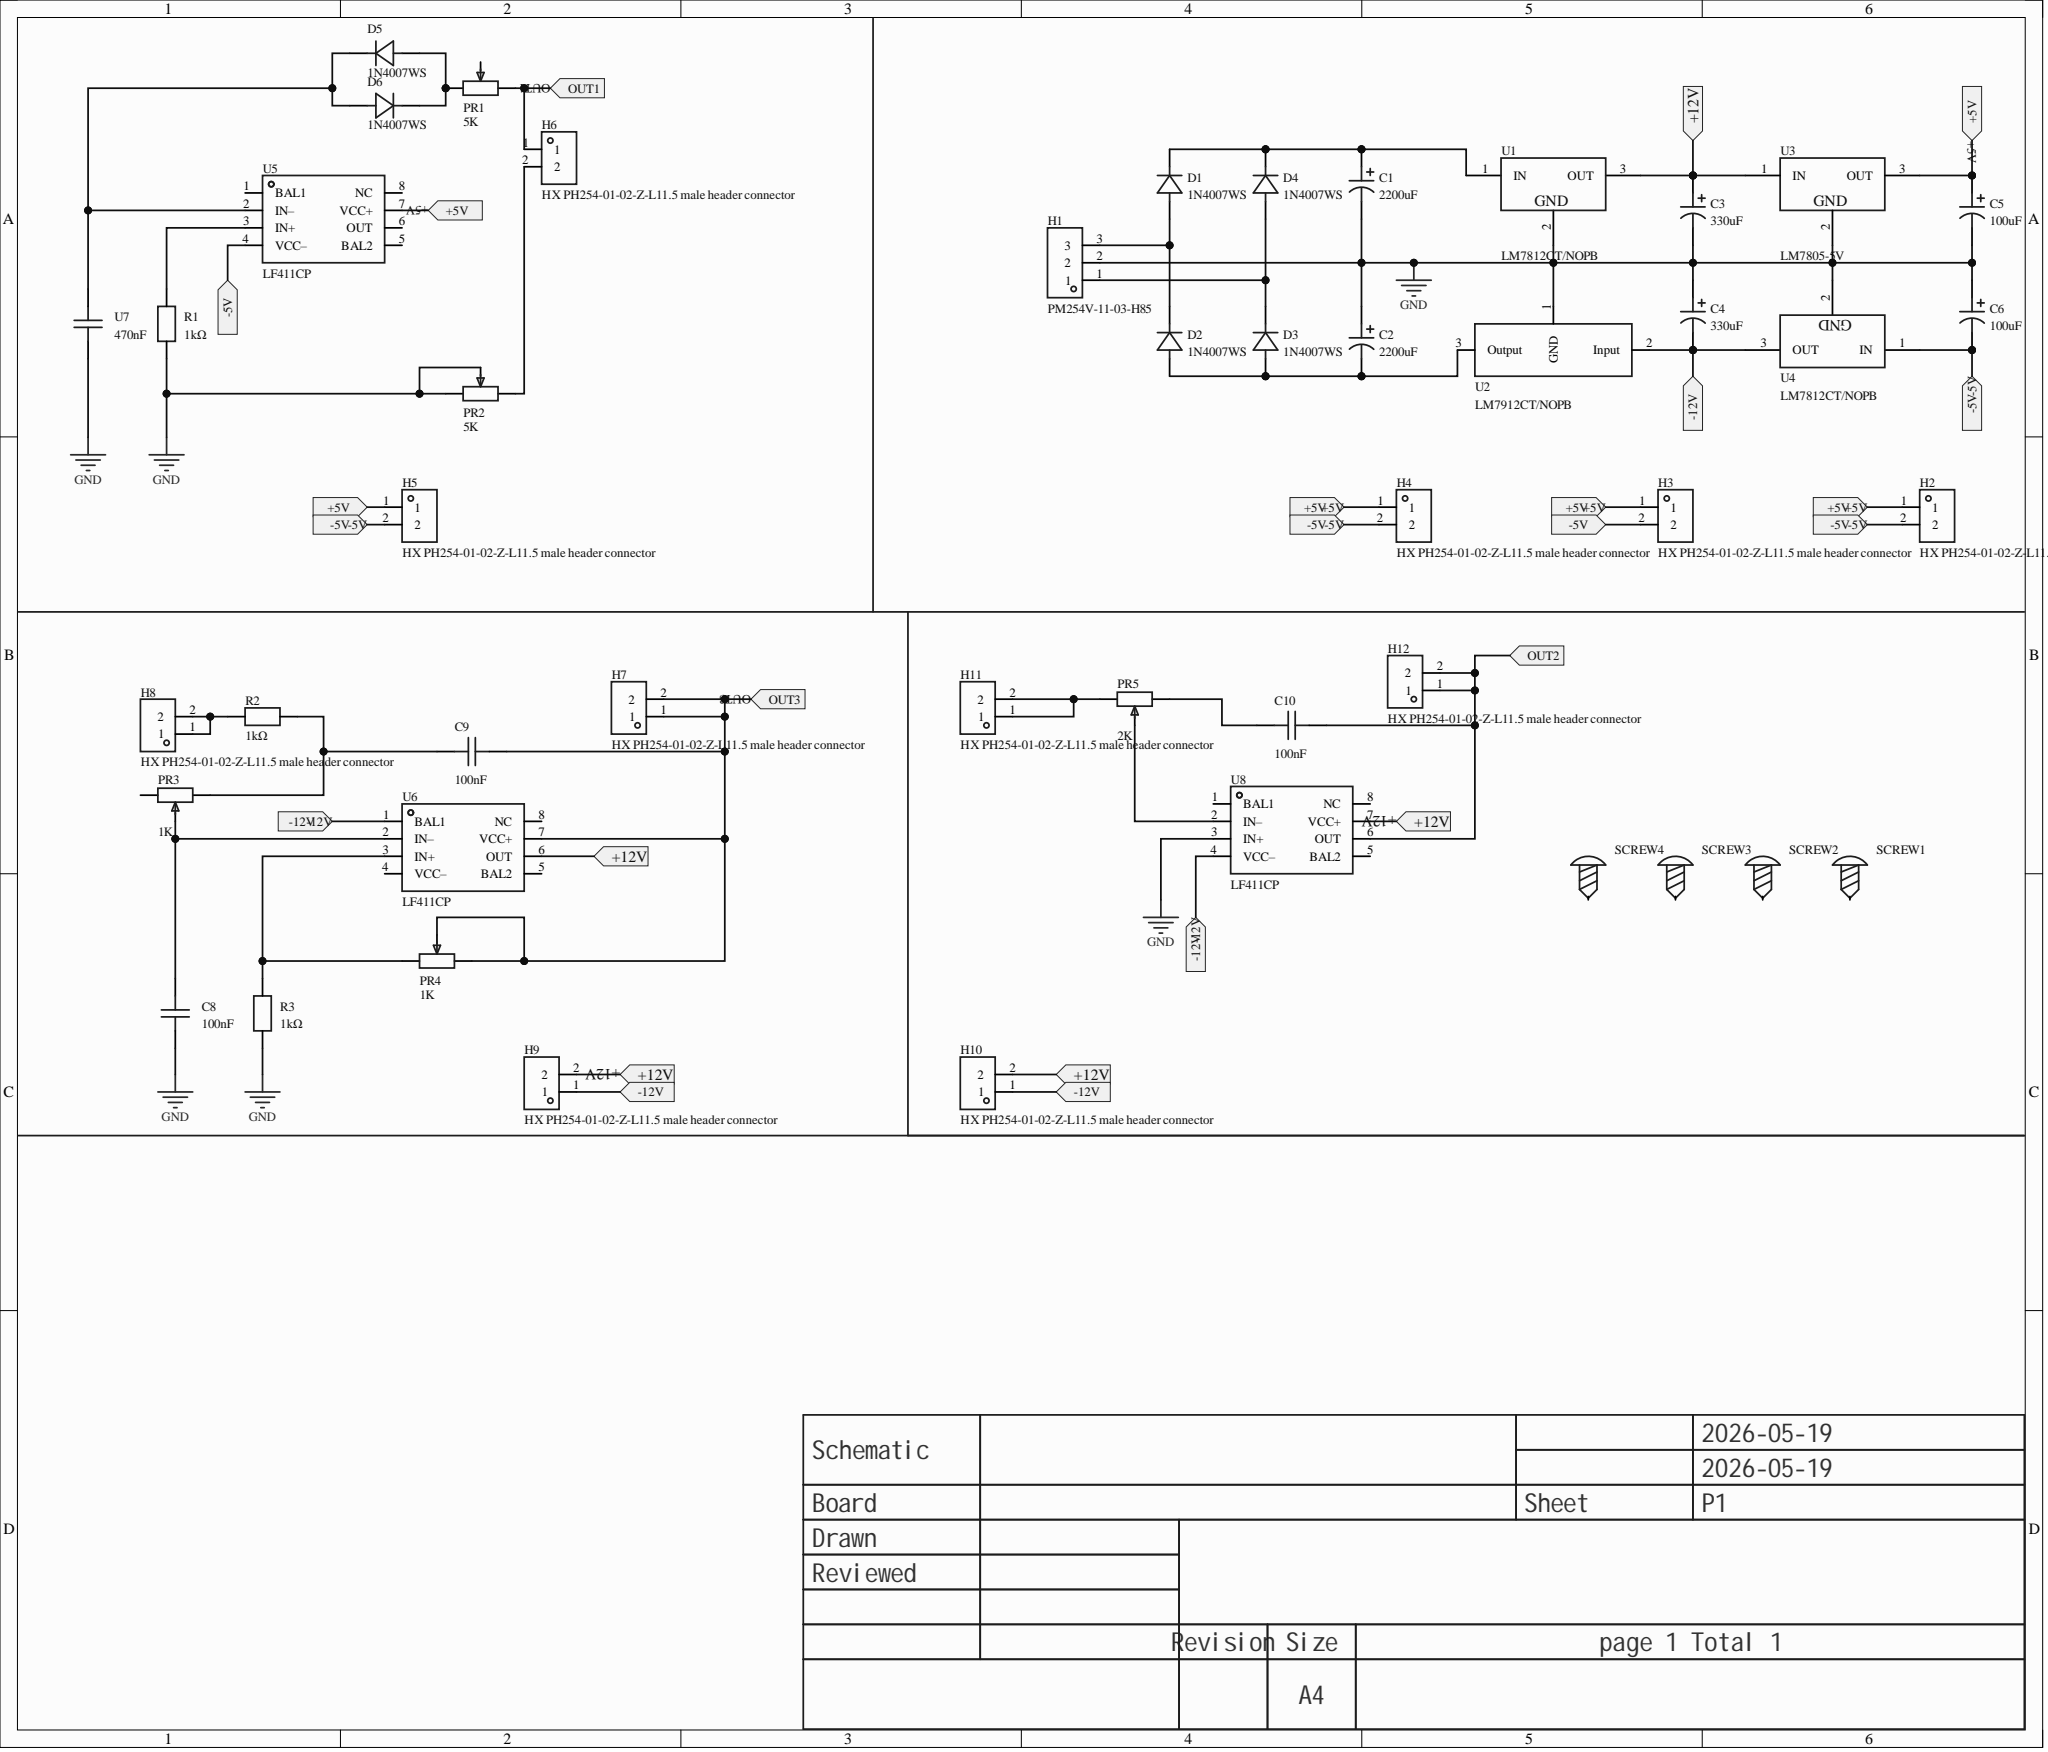Circuit board | Altium Designer | 47 parts | 23 nets
Bill of materials:
Comment,Description,Designator,Footprint,LibRef,Quantity
"2200uF","Capacitance:2200uF;Tolerance:±20%;Rated voltage:35V;","C1, C2","CAP-TH_BD16.0-P7.50-D0.8-FD","ERA35V2200M16X26","2"
"330uF","Capacitance:330uF;Tolerance:±20%;Rated voltage:16V;Ripple current:105mA@120Hz;Equivalent series resistance (ESR):-;","C3, C4","CAP-SMD_BD6.3-L6.6-W6.6-LS7.2-FD_3","RVT16V330M6X8","2"
"100uF","Capacitance:100uF;Tolerance:±20%;Rated voltage:50V;Ripple current:140mA@120Hz;","C5, C6","CAP-SMD_BD6.3-L6.6-W6.6-LS7.3-FD-H7.7","JVJ50V100M6x8","2"
"100nF","Capacitance:100nF;Tolerance:-20%~+80%;Rated voltage:50V;Temperature coefficient:Y5V;","C8, C9, C10","CAP-TH_L5.0-W2.5-P2.54-D0.7","CC1H104ZA1PD3F5P3003","3"
"1N4007WS","Diode configuration:1 single unit;Forward voltage (Vf):1.1V@1A;DC reverse voltage (Vr):1kV;Rectified current:1A;","D1, D2, D3, D4, D5, D6","SOD-323_L1.7-W1.3-LS2.5-RD","1N4007WS_C53055759","6"
"PM254V-11-03-H85","Socket structure:1x3P;Pitch:2.54mm;Row spacing:-;Round/square hole:Square hole;Mounting:Through-hole;Rows:Single row;Total holes:3P;Rated current:3A;Socket direction:Top;Plastic height:8.5mm;Contact material:Brass;Contact plating:-;Operating temperature:-40℃~+105℃;","H1","HDR-TH_3P-P2.54-V-F","PM254V-11-03-H85","1"
"HX PH254-01-02-Z-L11.5 male header connector","Pin structure:1x2P;Pitch:2.54mm;Round/square pin:Square pin;Mounting:Through-hole;Rows:Single row;Total pins:2P;Rated current:3A;Rated voltage:1kV;Mating pin length:6mm;Plastic height:2.5mm;Termination pin length:3mm;Contact material:Brass;Contact plating:Gold;Operating temperature:-40℃~+105℃;","H2, H3, H4, H5, H6, H7, H8, H9, H10, H11, H12","HDR-TH_2P-P2.54-V-M","HX PH254-01-02-Z-L11.5 male header connector","11"
"5K","","PR1, PR2","R_3386P","R_3386P","2"
"1K","","PR3, PR4","R_3386P","R_3386P","2"
"2K","","PR5","R_3386P","R_3386P","1"
"1kΩ","Resistor type:Thick film resistor;Resistance:1kΩ;Tolerance:±0.1%;Power:100mW;Working voltage:75V;Temperature coefficient:±100ppm/?;","R1, R2, R3","R0603","FRH0603B1001TS","3"
"","","SCREW1, SCREW2, SCREW3, SCREW4","M2螺丝","M2螺丝","4"
"LM7812CT/NOPB","Output type:Fixed;Max input voltage:-;Output voltage:12V;Output current:1.5A;Power supply rejection ratio (PSRR):72dB@(120Hz);Output polarity:Positive;","U1, U4","TO-220-3_L10.2-W4.6-P2.54-L","LM7812CT/NOPB","2"
"LM7912CT/NOPB","Output type:Fixed;Max input voltage:35V;Output voltage:12V;Output current:1.5A;Power supply rejection ratio (PSRR):70dB@(120Hz);Output polarity:Negative;","U2","TO-220-3_L10.2-W4.6-P2.54-L","LM7912CT/NOPB","1"
"LM7805-5V","","U3","TO-252-2_L6.6-W6.1-P4.58-LS9.9-TL","LM7805-5V_C9900008050","1"
"LF411CP","Gain-bandwidth product (GBP):3MHz;Input bias current (Ib):50pA;Input offset voltage (Vos):800uV;Slew rate (SR):13V/us;","U5, U6, U8","PDIP-8_L9.3-W6.4-P2.54-LS7.9-BL-1","LF411CP","3"
"470nF","Capacitance:470nF;Tolerance:±10%;Rated voltage:50V;Temperature coefficient:X7R;","U7","CAP-TH_L4.8-W2.4-P5.08-D0.6","178MU0009","1"
Netlist (Protel format):
[
C1
CAP-TH_BD16.0-P7.50-D0.8-FD
2200uF



]
[
C2
CAP-TH_BD16.0-P7.50-D0.8-FD
2200uF



]
[
C3
CAP-SMD_BD6.3-L6.6-W6.6-LS7.2-FD_3
330uF



]
[
C4
CAP-SMD_BD6.3-L6.6-W6.6-LS7.2-FD_3
330uF



]
[
C5
CAP-SMD_BD6.3-L6.6-W6.6-LS7.3-FD-H7.7
100uF



]
[
C6
CAP-SMD_BD6.3-L6.6-W6.6-LS7.3-FD-H7.7
100uF



]
[
C8
CAP-TH_L5.0-W2.5-P2.54-D0.7
100nF



]
[
C9
CAP-TH_L5.0-W2.5-P2.54-D0.7
100nF



]
[
C10
CAP-TH_L5.0-W2.5-P2.54-D0.7
100nF



]
[
D1
SOD-323_L1.7-W1.3-LS2.5-RD
1N4007WS



]
[
D2
SOD-323_L1.7-W1.3-LS2.5-RD
1N4007WS



]
[
D3
SOD-323_L1.7-W1.3-LS2.5-RD
1N4007WS



]
[
D4
SOD-323_L1.7-W1.3-LS2.5-RD
1N4007WS



]
[
D5
SOD-323_L1.7-W1.3-LS2.5-RD
1N4007WS



]
[
D6
SOD-323_L1.7-W1.3-LS2.5-RD
1N4007WS



]
[
H1
HDR-TH_3P-P2.54-V-F
PM254V-11-03-H85



]
[
H2
HDR-TH_2P-P2.54-V-M
HX PH254-01-02-Z-L11.5 male header connector



]
[
H3
HDR-TH_2P-P2.54-V-M
HX PH254-01-02-Z-L11.5 male header connector



]
[
H4
HDR-TH_2P-P2.54-V-M
HX PH254-01-02-Z-L11.5 male header connector



]
[
H5
HDR-TH_2P-P2.54-V-M
HX PH254-01-02-Z-L11.5 male header connector



]
[
H6
HDR-TH_2P-P2.54-V-M
HX PH254-01-02-Z-L11.5 male header connector



]
[
H7
HDR-TH_2P-P2.54-V-M
HX PH254-01-02-Z-L11.5 male header connector



]
[
H8
HDR-TH_2P-P2.54-V-M
HX PH254-01-02-Z-L11.5 male header connector



]
[
H9
HDR-TH_2P-P2.54-V-M
HX PH254-01-02-Z-L11.5 male header connector



]
[
H10
HDR-TH_2P-P2.54-V-M
HX PH254-01-02-Z-L11.5 male header connector



]
[
H11
HDR-TH_2P-P2.54-V-M
HX PH254-01-02-Z-L11.5 male header connector



]
[
H12
HDR-TH_2P-P2.54-V-M
HX PH254-01-02-Z-L11.5 male header connector



]
[
PR1
R_3386P
5K



]
[
PR2
R_3386P
5K



]
[
PR3
R_3386P
1K



]
[
PR4
R_3386P
1K



]
[
PR5
R_3386P
2K



]
[
R1
R0603
1kΩ



]
[
R2
R0603
1kΩ



]
[
R3
R0603
1kΩ



]
[
SCREW1
M2螺丝




]
[
SCREW2
M2螺丝




]
[
SCREW3
M2螺丝




]
[
SCREW4
M2螺丝




]
[
U1
TO-220-3_L10.2-W4.6-P2.54-L
LM7812CT/NOPB



]
[
U2
TO-220-3_L10.2-W4.6-P2.54-L
LM7912CT/NOPB



]
[
U3
TO-252-2_L6.6-W6.1-P4.58-LS9.9-TL
LM7805-5V



]
[
U4
TO-220-3_L10.2-W4.6-P2.54-L
LM7812CT/NOPB



]
[
U5
PDIP-8_L9.3-W6.4-P2.54-LS7.9-BL-1
LF411CP



]
[
U6
PDIP-8_L9.3-W6.4-P2.54-LS7.9-BL-1
LF411CP



]
[
U7
CAP-TH_L4.8-W2.4-P5.08-D0.6
470nF



]
[
U8
PDIP-8_L9.3-W6.4-P2.54-LS7.9-BL-1
LF411CP



]
(
OUT3
C9-2
H7-1
H7-2
PR4-1
PR4-2
U6-7
)
(
OUT1
H6-1
PR1-1
)
(
NetR1_2
R1-2
U5-3
)
(
NetPR5_2
PR5-2
U8-2
)
(
NetPR4_3
PR4-3
R3-2
U6-3
)
(
NetH11_1
H11-1
H11-2
PR5-1
)
(
NetH8_1
H8-1
H8-2
R2-1
)
(
NetH6_2
H6-2
PR2-1
)
(
NetD5_2
D5-2
D6-1
PR1-3
)
(
NetD5_1
D5-1
D6-2
U5-2
U7-2
)
(
NetD3_1
D3-1
D4-2
H1-1
)
(
NetD1_2
D1-2
D2-1
H1-3
)
(
NetC10_2
C10-2
H12-1
H12-2
U8-6
)
(
NetC10_1
C10-1
PR5-3
)
(
NetC9_1
C9-1
PR3-3
R2-2
)
(
NetC8_1
C8-1
PR3-2
U6-2
)
(
NetC2_2
C2-2
D2-2
D3-2
U2-3
)
(
NetC1_1
C1-1
D1-1
D4-1
U1-1
)
(
GND
C1-2
C2-1
C3-2
C4-1
C5-2
C6-1
C8-2
H1-2
PR2-2
PR2-3
R1-1
R3-1
U1-2
U2-1
U3-2
U4-2
U7-1
U8-3
)
(
-12V
C4-2
H9-1
H10-1
U2-2
U4-3
U6-1
U8-4
)
(
-5V
C6-2
H2-2
H3-2
H4-2
H5-2
U4-1
U5-4
)
(
+12V
C3-1
H9-2
H10-2
U1-3
U3-1
U6-6
U8-7
)
(
+5V
C5-1
H2-1
H3-1
H4-1
H5-1
U3-3
U5-7
)